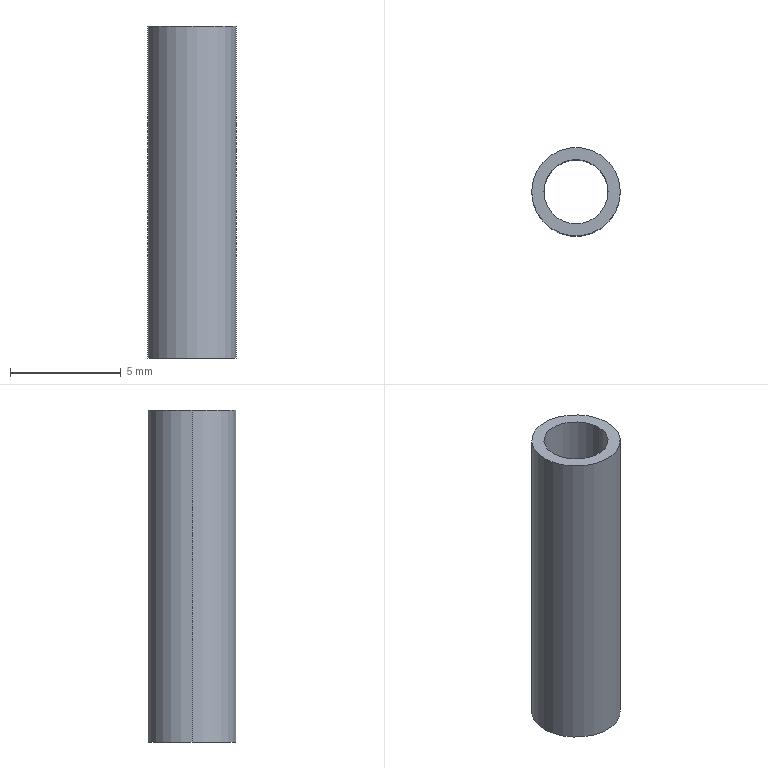Part | STEP file | UM4-15 | 1 solid | 6 faces | box 4 x 4 x 15 mm | volume 89.418 mm3 | cylinder 4 | plane 2 | commonest cylinder face diameters 2.9 x2 4 x2
STEP:
#1=CARTESIAN_POINT('',(0.,0.,0.));
#2=DIRECTION('',(0.,0.,1.));
#3=DIRECTION('',(1.,0.,0.));
#4=AXIS2_PLACEMENT_3D('',#1,#2,#3);
#5=CARTESIAN_POINT('',(-1.45,0.,15.));
#6=VERTEX_POINT('',#5);
#7=CARTESIAN_POINT('',(-1.45,0.,0.));
#8=VERTEX_POINT('',#7);
#9=CARTESIAN_POINT('',(-1.45,0.,15.));
#10=DIRECTION('',(0.,0.,-1.));
#11=VECTOR('',#10,1.);
#12=LINE('',#9,#11);
#13=CARTESIAN_POINT('',(0.,0.,15.));
#14=DIRECTION('',(0.,0.,-1.));
#15=DIRECTION('',(-1.,0.,0.));
#16=AXIS2_PLACEMENT_3D('',#13,#14,#15);
#17=CYLINDRICAL_SURFACE('',#16,1.45);
#18=CARTESIAN_POINT('',(6.283,0.));
#19=DIRECTION('',(0.,1.));
#20=VECTOR('',#19,1.);
#21=LINE('',#18,#20);
#22=(GEOMETRIC_REPRESENTATION_CONTEXT(2)PARAMETRIC_REPRESENTATION_CONTEXT()REPRESENTATION_CONTEXT('',''));
#23=DEFINITIONAL_REPRESENTATION('',(#21),#22);
#24=PCURVE('',#17,#23);
#25=CARTESIAN_POINT('',(0.,0.,15.));
#26=DIRECTION('',(0.,0.,-1.));
#27=DIRECTION('',(-1.,0.,0.));
#28=AXIS2_PLACEMENT_3D('',#25,#26,#27);
#29=CYLINDRICAL_SURFACE('',#28,1.45);
#30=CARTESIAN_POINT('',(0.,0.));
#31=DIRECTION('',(0.,1.));
#32=VECTOR('',#31,1.);
#33=LINE('',#30,#32);
#34=(GEOMETRIC_REPRESENTATION_CONTEXT(2)PARAMETRIC_REPRESENTATION_CONTEXT()REPRESENTATION_CONTEXT('',''));
#35=DEFINITIONAL_REPRESENTATION('',(#33),#34);
#36=PCURVE('',#29,#35);
#37=SURFACE_CURVE('',#12,(#24,#36),.PCURVE_S1.);
#38=EDGE_CURVE('',#6,#8,#37,.T.);
#39=ORIENTED_EDGE('',*,*,#38,.T.);
#40=CARTESIAN_POINT('',(1.45,0.,0.));
#41=VERTEX_POINT('',#40);
#42=CARTESIAN_POINT('',(0.,0.,0.));
#43=DIRECTION('',(0.,0.,1.));
#44=DIRECTION('',(1.,0.,0.));
#45=AXIS2_PLACEMENT_3D('',#42,#43,#44);
#46=CIRCLE('',#45,1.45);
#47=CARTESIAN_POINT('',(9.425,15.));
#48=DIRECTION('',(-1.,0.));
#49=VECTOR('',#48,1.);
#50=LINE('',#47,#49);
#51=(GEOMETRIC_REPRESENTATION_CONTEXT(2)PARAMETRIC_REPRESENTATION_CONTEXT()REPRESENTATION_CONTEXT('',''));
#52=DEFINITIONAL_REPRESENTATION('',(#50),#51);
#53=PCURVE('',#17,#52);
#54=CARTESIAN_POINT('',(0.,0.,0.));
#55=DIRECTION('',(0.,0.,1.));
#56=DIRECTION('',(1.,0.,0.));
#57=AXIS2_PLACEMENT_3D('',#54,#55,#56);
#58=PLANE('',#57);
#59=CARTESIAN_POINT('',(0.,0.));
#60=DIRECTION('',(1.,0.));
#61=AXIS2_PLACEMENT_2D('',#59,#60);
#62=CIRCLE('',#61,1.45);
#63=(GEOMETRIC_REPRESENTATION_CONTEXT(2)PARAMETRIC_REPRESENTATION_CONTEXT()REPRESENTATION_CONTEXT('',''));
#64=DEFINITIONAL_REPRESENTATION('',(#62),#63);
#65=PCURVE('',#58,#64);
#66=SURFACE_CURVE('',#46,(#53,#65),.PCURVE_S1.);
#67=EDGE_CURVE('',#8,#41,#66,.T.);
#68=ORIENTED_EDGE('',*,*,#67,.T.);
#69=CARTESIAN_POINT('',(1.45,0.,15.));
#70=VERTEX_POINT('',#69);
#71=CARTESIAN_POINT('',(1.45,0.,15.));
#72=DIRECTION('',(0.,0.,-1.));
#73=VECTOR('',#72,1.);
#74=LINE('',#71,#73);
#75=CARTESIAN_POINT('',(3.142,0.));
#76=DIRECTION('',(0.,1.));
#77=VECTOR('',#76,1.);
#78=LINE('',#75,#77);
#79=(GEOMETRIC_REPRESENTATION_CONTEXT(2)PARAMETRIC_REPRESENTATION_CONTEXT()REPRESENTATION_CONTEXT('',''));
#80=DEFINITIONAL_REPRESENTATION('',(#78),#79);
#81=PCURVE('',#17,#80);
#82=CARTESIAN_POINT('',(3.142,0.));
#83=DIRECTION('',(0.,1.));
#84=VECTOR('',#83,1.);
#85=LINE('',#82,#84);
#86=(GEOMETRIC_REPRESENTATION_CONTEXT(2)PARAMETRIC_REPRESENTATION_CONTEXT()REPRESENTATION_CONTEXT('',''));
#87=DEFINITIONAL_REPRESENTATION('',(#85),#86);
#88=PCURVE('',#29,#87);
#89=SURFACE_CURVE('',#74,(#81,#88),.PCURVE_S1.);
#90=EDGE_CURVE('',#70,#41,#89,.T.);
#91=ORIENTED_EDGE('',*,*,#90,.F.);
#92=CARTESIAN_POINT('',(0.,0.,15.));
#93=DIRECTION('',(0.,0.,1.));
#94=DIRECTION('',(1.,0.,0.));
#95=AXIS2_PLACEMENT_3D('',#92,#93,#94);
#96=CIRCLE('',#95,1.45);
#97=CARTESIAN_POINT('',(9.425,0.));
#98=DIRECTION('',(-1.,0.));
#99=VECTOR('',#98,1.);
#100=LINE('',#97,#99);
#101=(GEOMETRIC_REPRESENTATION_CONTEXT(2)PARAMETRIC_REPRESENTATION_CONTEXT()REPRESENTATION_CONTEXT('',''));
#102=DEFINITIONAL_REPRESENTATION('',(#100),#101);
#103=PCURVE('',#17,#102);
#104=CARTESIAN_POINT('',(0.,0.,15.));
#105=DIRECTION('',(0.,0.,1.));
#106=DIRECTION('',(1.,0.,0.));
#107=AXIS2_PLACEMENT_3D('',#104,#105,#106);
#108=PLANE('',#107);
#109=CARTESIAN_POINT('',(0.,0.));
#110=DIRECTION('',(1.,0.));
#111=AXIS2_PLACEMENT_2D('',#109,#110);
#112=CIRCLE('',#111,1.45);
#113=(GEOMETRIC_REPRESENTATION_CONTEXT(2)PARAMETRIC_REPRESENTATION_CONTEXT()REPRESENTATION_CONTEXT('',''));
#114=DEFINITIONAL_REPRESENTATION('',(#112),#113);
#115=PCURVE('',#108,#114);
#116=SURFACE_CURVE('',#96,(#103,#115),.PCURVE_S1.);
#117=EDGE_CURVE('',#6,#70,#116,.T.);
#118=ORIENTED_EDGE('',*,*,#117,.F.);
#119=EDGE_LOOP('',(#39,#68,#91,#118));
#120=FACE_BOUND('',#119,.F.);
#121=ADVANCED_FACE('',(#120),#17,.F.);
#122=CARTESIAN_POINT('',(2.,0.,15.));
#123=VERTEX_POINT('',#122);
#124=CARTESIAN_POINT('',(-2.,0.,15.));
#125=VERTEX_POINT('',#124);
#126=CARTESIAN_POINT('',(0.,0.,15.));
#127=DIRECTION('',(0.,0.,1.));
#128=DIRECTION('',(1.,0.,0.));
#129=AXIS2_PLACEMENT_3D('',#126,#127,#128);
#130=CIRCLE('',#129,2.);
#131=CARTESIAN_POINT('',(0.,0.,15.));
#132=DIRECTION('',(0.,0.,-1.));
#133=DIRECTION('',(-1.,0.,0.));
#134=AXIS2_PLACEMENT_3D('',#131,#132,#133);
#135=CYLINDRICAL_SURFACE('',#134,2.);
#136=CARTESIAN_POINT('',(3.142,0.));
#137=DIRECTION('',(-1.,0.));
#138=VECTOR('',#137,1.);
#139=LINE('',#136,#138);
#140=(GEOMETRIC_REPRESENTATION_CONTEXT(2)PARAMETRIC_REPRESENTATION_CONTEXT()REPRESENTATION_CONTEXT('',''));
#141=DEFINITIONAL_REPRESENTATION('',(#139),#140);
#142=PCURVE('',#135,#141);
#143=CARTESIAN_POINT('',(0.,0.));
#144=DIRECTION('',(1.,0.));
#145=AXIS2_PLACEMENT_2D('',#143,#144);
#146=CIRCLE('',#145,2.);
#147=(GEOMETRIC_REPRESENTATION_CONTEXT(2)PARAMETRIC_REPRESENTATION_CONTEXT()REPRESENTATION_CONTEXT('',''));
#148=DEFINITIONAL_REPRESENTATION('',(#146),#147);
#149=PCURVE('',#108,#148);
#150=SURFACE_CURVE('',#130,(#142,#149),.PCURVE_S1.);
#151=EDGE_CURVE('',#123,#125,#150,.T.);
#152=ORIENTED_EDGE('',*,*,#151,.F.);
#153=CARTESIAN_POINT('',(2.,0.,0.));
#154=VERTEX_POINT('',#153);
#155=CARTESIAN_POINT('',(2.,0.,15.));
#156=DIRECTION('',(0.,0.,-1.));
#157=VECTOR('',#156,1.);
#158=LINE('',#155,#157);
#159=CARTESIAN_POINT('',(3.142,0.));
#160=DIRECTION('',(0.,1.));
#161=VECTOR('',#160,1.);
#162=LINE('',#159,#161);
#163=(GEOMETRIC_REPRESENTATION_CONTEXT(2)PARAMETRIC_REPRESENTATION_CONTEXT()REPRESENTATION_CONTEXT('',''));
#164=DEFINITIONAL_REPRESENTATION('',(#162),#163);
#165=PCURVE('',#135,#164);
#166=CARTESIAN_POINT('',(0.,0.,15.));
#167=DIRECTION('',(0.,0.,-1.));
#168=DIRECTION('',(-1.,0.,0.));
#169=AXIS2_PLACEMENT_3D('',#166,#167,#168);
#170=CYLINDRICAL_SURFACE('',#169,2.);
#171=CARTESIAN_POINT('',(3.142,0.));
#172=DIRECTION('',(0.,1.));
#173=VECTOR('',#172,1.);
#174=LINE('',#171,#173);
#175=(GEOMETRIC_REPRESENTATION_CONTEXT(2)PARAMETRIC_REPRESENTATION_CONTEXT()REPRESENTATION_CONTEXT('',''));
#176=DEFINITIONAL_REPRESENTATION('',(#174),#175);
#177=PCURVE('',#170,#176);
#178=SURFACE_CURVE('',#158,(#165,#177),.PCURVE_S1.);
#179=EDGE_CURVE('',#123,#154,#178,.T.);
#180=ORIENTED_EDGE('',*,*,#179,.T.);
#181=CARTESIAN_POINT('',(-2.,0.,0.));
#182=VERTEX_POINT('',#181);
#183=CARTESIAN_POINT('',(0.,0.,0.));
#184=DIRECTION('',(0.,0.,1.));
#185=DIRECTION('',(1.,0.,0.));
#186=AXIS2_PLACEMENT_3D('',#183,#184,#185);
#187=CIRCLE('',#186,2.);
#188=CARTESIAN_POINT('',(3.142,15.));
#189=DIRECTION('',(-1.,0.));
#190=VECTOR('',#189,1.);
#191=LINE('',#188,#190);
#192=(GEOMETRIC_REPRESENTATION_CONTEXT(2)PARAMETRIC_REPRESENTATION_CONTEXT()REPRESENTATION_CONTEXT('',''));
#193=DEFINITIONAL_REPRESENTATION('',(#191),#192);
#194=PCURVE('',#135,#193);
#195=CARTESIAN_POINT('',(0.,0.));
#196=DIRECTION('',(1.,0.));
#197=AXIS2_PLACEMENT_2D('',#195,#196);
#198=CIRCLE('',#197,2.);
#199=(GEOMETRIC_REPRESENTATION_CONTEXT(2)PARAMETRIC_REPRESENTATION_CONTEXT()REPRESENTATION_CONTEXT('',''));
#200=DEFINITIONAL_REPRESENTATION('',(#198),#199);
#201=PCURVE('',#58,#200);
#202=SURFACE_CURVE('',#187,(#194,#201),.PCURVE_S1.);
#203=EDGE_CURVE('',#154,#182,#202,.T.);
#204=ORIENTED_EDGE('',*,*,#203,.T.);
#205=CARTESIAN_POINT('',(-2.,0.,15.));
#206=DIRECTION('',(0.,0.,-1.));
#207=VECTOR('',#206,1.);
#208=LINE('',#205,#207);
#209=CARTESIAN_POINT('',(0.,0.));
#210=DIRECTION('',(0.,1.));
#211=VECTOR('',#210,1.);
#212=LINE('',#209,#211);
#213=(GEOMETRIC_REPRESENTATION_CONTEXT(2)PARAMETRIC_REPRESENTATION_CONTEXT()REPRESENTATION_CONTEXT('',''));
#214=DEFINITIONAL_REPRESENTATION('',(#212),#213);
#215=PCURVE('',#135,#214);
#216=CARTESIAN_POINT('',(6.283,0.));
#217=DIRECTION('',(0.,1.));
#218=VECTOR('',#217,1.);
#219=LINE('',#216,#218);
#220=(GEOMETRIC_REPRESENTATION_CONTEXT(2)PARAMETRIC_REPRESENTATION_CONTEXT()REPRESENTATION_CONTEXT('',''));
#221=DEFINITIONAL_REPRESENTATION('',(#219),#220);
#222=PCURVE('',#170,#221);
#223=SURFACE_CURVE('',#208,(#215,#222),.PCURVE_S1.);
#224=EDGE_CURVE('',#125,#182,#223,.T.);
#225=ORIENTED_EDGE('',*,*,#224,.F.);
#226=EDGE_LOOP('',(#152,#180,#204,#225));
#227=FACE_BOUND('',#226,.T.);
#228=ADVANCED_FACE('',(#227),#135,.T.);
#229=CARTESIAN_POINT('',(0.,0.,15.));
#230=DIRECTION('',(0.,0.,1.));
#231=DIRECTION('',(1.,0.,0.));
#232=AXIS2_PLACEMENT_3D('',#229,#230,#231);
#233=CIRCLE('',#232,2.);
#234=CARTESIAN_POINT('',(0.,0.));
#235=DIRECTION('',(1.,0.));
#236=AXIS2_PLACEMENT_2D('',#234,#235);
#237=CIRCLE('',#236,2.);
#238=(GEOMETRIC_REPRESENTATION_CONTEXT(2)PARAMETRIC_REPRESENTATION_CONTEXT()REPRESENTATION_CONTEXT('',''));
#239=DEFINITIONAL_REPRESENTATION('',(#237),#238);
#240=PCURVE('',#108,#239);
#241=CARTESIAN_POINT('',(9.425,0.));
#242=DIRECTION('',(-1.,0.));
#243=VECTOR('',#242,1.);
#244=LINE('',#241,#243);
#245=(GEOMETRIC_REPRESENTATION_CONTEXT(2)PARAMETRIC_REPRESENTATION_CONTEXT()REPRESENTATION_CONTEXT('',''));
#246=DEFINITIONAL_REPRESENTATION('',(#244),#245);
#247=PCURVE('',#170,#246);
#248=SURFACE_CURVE('',#233,(#240,#247),.PCURVE_S1.);
#249=EDGE_CURVE('',#125,#123,#248,.T.);
#250=ORIENTED_EDGE('',*,*,#249,.T.);
#251=ORIENTED_EDGE('',*,*,#151,.T.);
#252=EDGE_LOOP('',(#250,#251));
#253=FACE_BOUND('',#252,.T.);
#254=ORIENTED_EDGE('',*,*,#117,.F.);
#255=CARTESIAN_POINT('',(0.,0.,15.));
#256=DIRECTION('',(0.,0.,1.));
#257=DIRECTION('',(1.,0.,0.));
#258=AXIS2_PLACEMENT_3D('',#255,#256,#257);
#259=CIRCLE('',#258,1.45);
#260=CARTESIAN_POINT('',(0.,0.));
#261=DIRECTION('',(1.,0.));
#262=AXIS2_PLACEMENT_2D('',#260,#261);
#263=CIRCLE('',#262,1.45);
#264=(GEOMETRIC_REPRESENTATION_CONTEXT(2)PARAMETRIC_REPRESENTATION_CONTEXT()REPRESENTATION_CONTEXT('',''));
#265=DEFINITIONAL_REPRESENTATION('',(#263),#264);
#266=PCURVE('',#108,#265);
#267=CARTESIAN_POINT('',(3.142,0.));
#268=DIRECTION('',(-1.,0.));
#269=VECTOR('',#268,1.);
#270=LINE('',#267,#269);
#271=(GEOMETRIC_REPRESENTATION_CONTEXT(2)PARAMETRIC_REPRESENTATION_CONTEXT()REPRESENTATION_CONTEXT('',''));
#272=DEFINITIONAL_REPRESENTATION('',(#270),#271);
#273=PCURVE('',#29,#272);
#274=SURFACE_CURVE('',#259,(#266,#273),.PCURVE_S1.);
#275=EDGE_CURVE('',#70,#6,#274,.T.);
#276=ORIENTED_EDGE('',*,*,#275,.F.);
#277=EDGE_LOOP('',(#254,#276));
#278=FACE_BOUND('',#277,.T.);
#279=ADVANCED_FACE('',(#253,#278),#108,.T.);
#280=CARTESIAN_POINT('',(0.,0.,0.));
#281=DIRECTION('',(0.,0.,1.));
#282=DIRECTION('',(1.,0.,0.));
#283=AXIS2_PLACEMENT_3D('',#280,#281,#282);
#284=CIRCLE('',#283,2.);
#285=CARTESIAN_POINT('',(0.,0.));
#286=DIRECTION('',(1.,0.));
#287=AXIS2_PLACEMENT_2D('',#285,#286);
#288=CIRCLE('',#287,2.);
#289=(GEOMETRIC_REPRESENTATION_CONTEXT(2)PARAMETRIC_REPRESENTATION_CONTEXT()REPRESENTATION_CONTEXT('',''));
#290=DEFINITIONAL_REPRESENTATION('',(#288),#289);
#291=PCURVE('',#58,#290);
#292=CARTESIAN_POINT('',(9.425,15.));
#293=DIRECTION('',(-1.,0.));
#294=VECTOR('',#293,1.);
#295=LINE('',#292,#294);
#296=(GEOMETRIC_REPRESENTATION_CONTEXT(2)PARAMETRIC_REPRESENTATION_CONTEXT()REPRESENTATION_CONTEXT('',''));
#297=DEFINITIONAL_REPRESENTATION('',(#295),#296);
#298=PCURVE('',#170,#297);
#299=SURFACE_CURVE('',#284,(#291,#298),.PCURVE_S1.);
#300=EDGE_CURVE('',#182,#154,#299,.T.);
#301=ORIENTED_EDGE('',*,*,#300,.F.);
#302=ORIENTED_EDGE('',*,*,#203,.F.);
#303=EDGE_LOOP('',(#301,#302));
#304=FACE_BOUND('',#303,.T.);
#305=ORIENTED_EDGE('',*,*,#67,.T.);
#306=CARTESIAN_POINT('',(0.,0.,0.));
#307=DIRECTION('',(0.,0.,1.));
#308=DIRECTION('',(1.,0.,0.));
#309=AXIS2_PLACEMENT_3D('',#306,#307,#308);
#310=CIRCLE('',#309,1.45);
#311=CARTESIAN_POINT('',(0.,0.));
#312=DIRECTION('',(1.,0.));
#313=AXIS2_PLACEMENT_2D('',#311,#312);
#314=CIRCLE('',#313,1.45);
#315=(GEOMETRIC_REPRESENTATION_CONTEXT(2)PARAMETRIC_REPRESENTATION_CONTEXT()REPRESENTATION_CONTEXT('',''));
#316=DEFINITIONAL_REPRESENTATION('',(#314),#315);
#317=PCURVE('',#58,#316);
#318=CARTESIAN_POINT('',(3.142,15.));
#319=DIRECTION('',(-1.,0.));
#320=VECTOR('',#319,1.);
#321=LINE('',#318,#320);
#322=(GEOMETRIC_REPRESENTATION_CONTEXT(2)PARAMETRIC_REPRESENTATION_CONTEXT()REPRESENTATION_CONTEXT('',''));
#323=DEFINITIONAL_REPRESENTATION('',(#321),#322);
#324=PCURVE('',#29,#323);
#325=SURFACE_CURVE('',#310,(#317,#324),.PCURVE_S1.);
#326=EDGE_CURVE('',#41,#8,#325,.T.);
#327=ORIENTED_EDGE('',*,*,#326,.T.);
#328=EDGE_LOOP('',(#305,#327));
#329=FACE_BOUND('',#328,.T.);
#330=ADVANCED_FACE('',(#304,#329),#58,.F.);
#331=ORIENTED_EDGE('',*,*,#179,.F.);
#332=ORIENTED_EDGE('',*,*,#249,.F.);
#333=ORIENTED_EDGE('',*,*,#224,.T.);
#334=ORIENTED_EDGE('',*,*,#300,.T.);
#335=EDGE_LOOP('',(#331,#332,#333,#334));
#336=FACE_BOUND('',#335,.T.);
#337=ADVANCED_FACE('',(#336),#170,.T.);
#338=ORIENTED_EDGE('',*,*,#326,.T.);
#339=ORIENTED_EDGE('',*,*,#38,.F.);
#340=ORIENTED_EDGE('',*,*,#275,.F.);
#341=ORIENTED_EDGE('',*,*,#90,.T.);
#342=EDGE_LOOP('',(#338,#339,#340,#341));
#343=FACE_BOUND('',#342,.F.);
#344=ADVANCED_FACE('',(#343),#29,.F.);
#345=CLOSED_SHELL('',(#121,#228,#279,#330,#337,#344));
#346=MANIFOLD_SOLID_BREP('',#345);
#347=(LENGTH_UNIT()NAMED_UNIT(*)SI_UNIT(.MILLI.,.METRE.));
#348=UNCERTAINTY_MEASURE_WITH_UNIT(LENGTH_MEASURE(0.0000001),#347,'','');
#349=(NAMED_UNIT(*)PLANE_ANGLE_UNIT()SI_UNIT($,.RADIAN.));
#350=(NAMED_UNIT(*)SI_UNIT($,.STERADIAN.)SOLID_ANGLE_UNIT());
#351=(GEOMETRIC_REPRESENTATION_CONTEXT(3)GLOBAL_UNCERTAINTY_ASSIGNED_CONTEXT((#348))GLOBAL_UNIT_ASSIGNED_CONTEXT((#347,#349,#350))REPRESENTATION_CONTEXT('',''));
#352=ADVANCED_BREP_SHAPE_REPRESENTATION('',(#4,#346),#351);